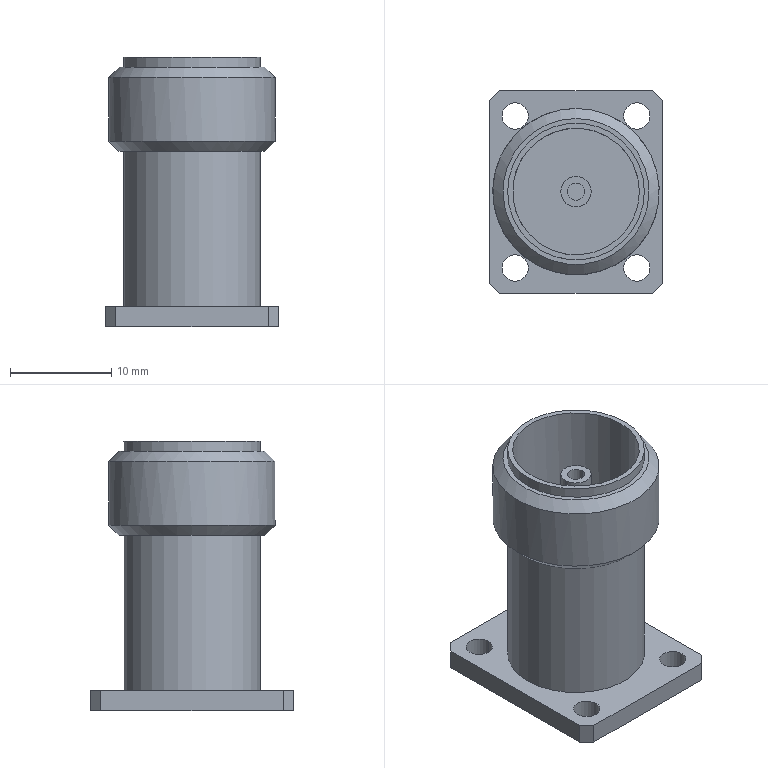Part | STEP file | Connector N-KFD612 | 1 solid | 34 faces | box 17 x 20 x 26.6 mm | volume 3584 mm3 | plane 17 | cylinder 15 | cone 2 | commonest cylinder face diameters 2.6 x5 1.7 x4 3 x2 13.5 x2 12.5 x1 16.413 x1